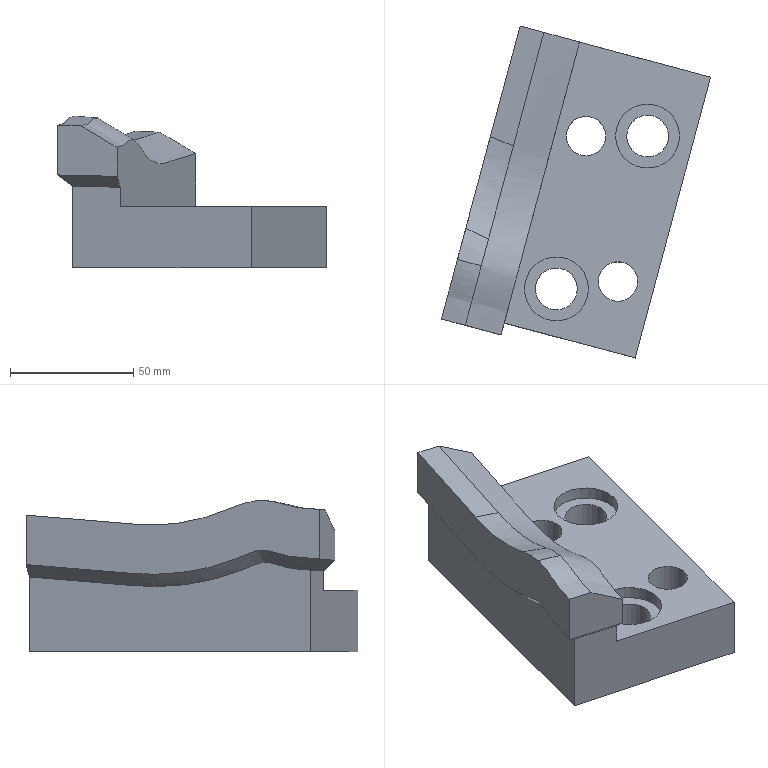Part | NX | features solid 2 | 1 solid | 24 faces | box 109.121 x 134.588 x 61.655 mm | volume 275417 mm3 | plane 10 | spline 8 | cylinder 6 | commonest cylinder face diameters 16 x2 17 x2 26 x2